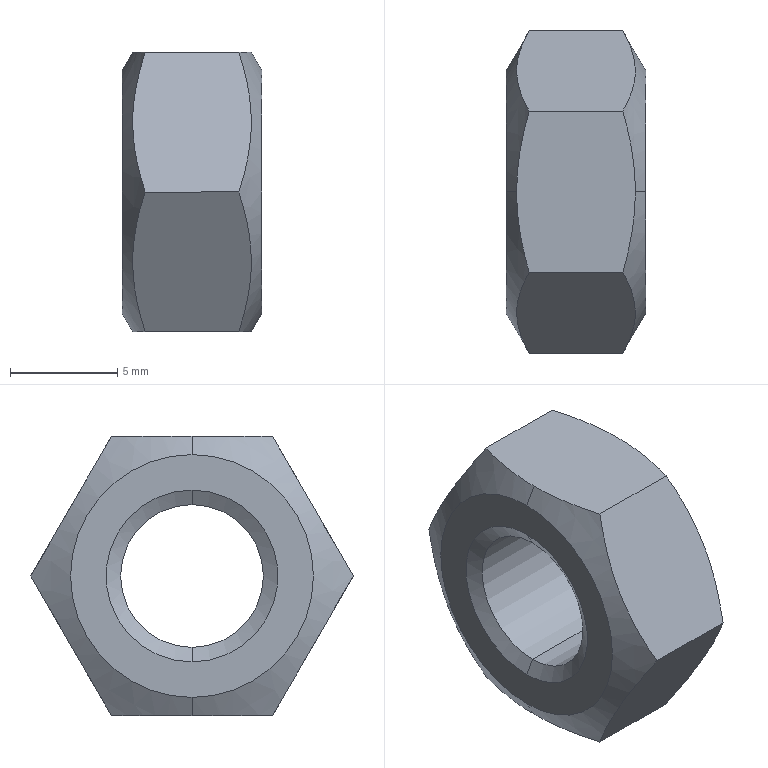Part | STEP file | DIN 934 - M8 x 1,25 | 1 solid | 18 faces | box 6.5 x 15.011 x 13 mm | volume 685.44 mm3 | cone 8 | plane 8 | cylinder 2 | commonest cylinder face diameters 6.647 x2